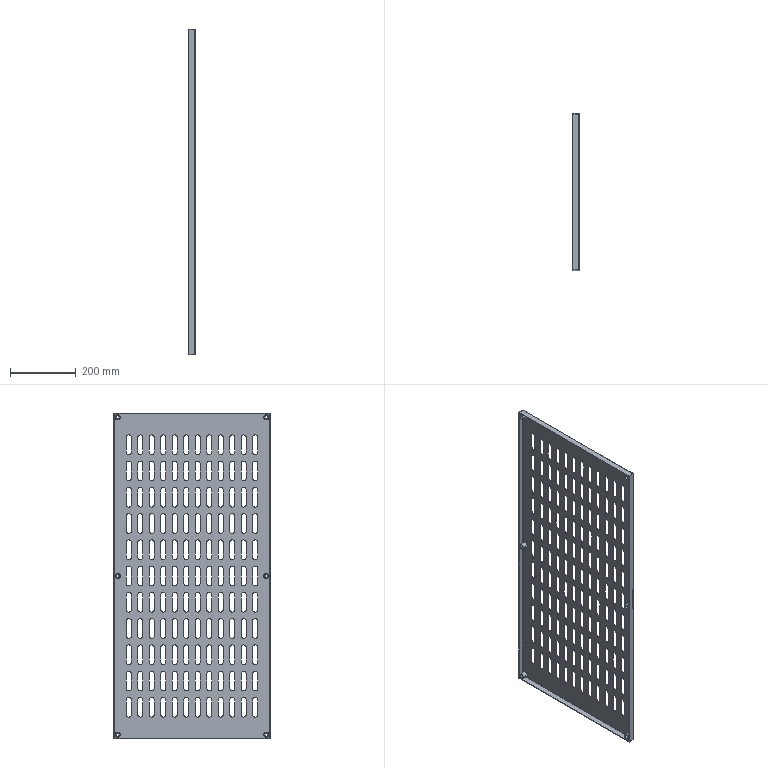Part | SolidWorks | 7 solids | 614 faces | box 19 x 477 x 992 mm | volume 830075 mm3 | cylinder 308 | plane 302 | spline 4 | commonest cylinder face diameters 15 x264 9 x12 10 x12 16 x12 0.2 x4 4.2 x4